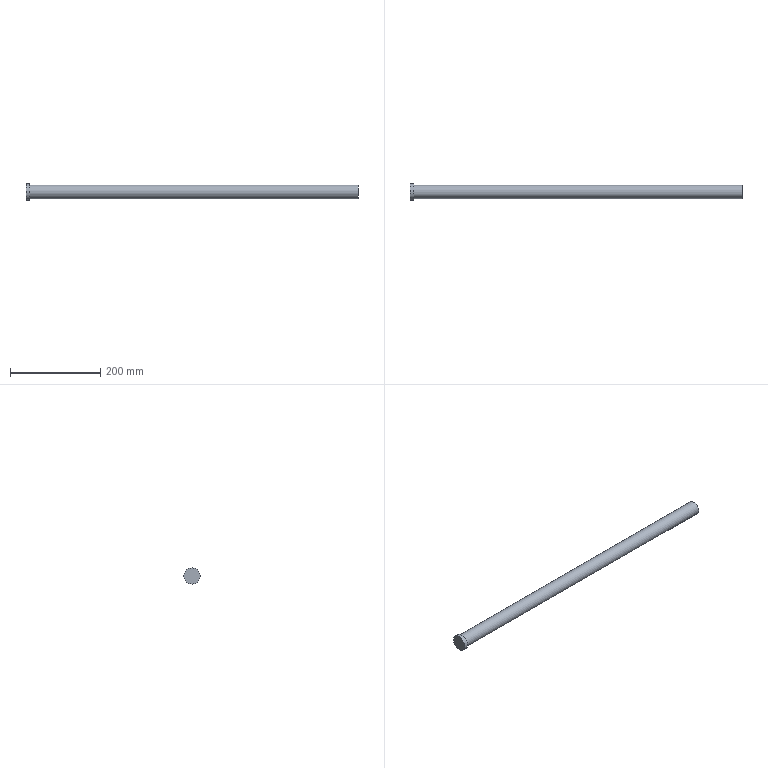Part | STEP file | solid 72 | 1 solid | 8 faces | box 736 x 36 x 36 mm | volume 520571 mm3 | plane 4 | cylinder 3 | cone 1 | commonest cylinder face diameters 10.5 x1 30 x1 36 x1